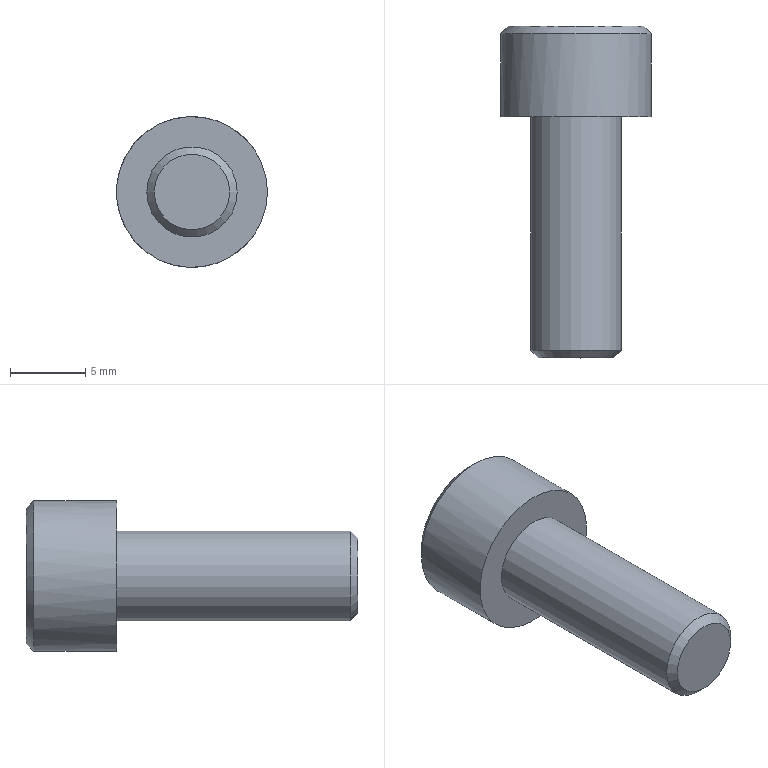Part | STEP file | gslz 2016.10.28-6_id710_x_t | 1 solid | 14 faces | box 10 x 22 x 10 mm | volume 831.004 mm3 | plane 10 | cylinder 2 | cone 2 | commonest cylinder face diameters 6 x1 10 x1
STEP:
#1=CARTESIAN_POINT('',(102.7,216.01,67.));
#2=VERTEX_POINT('',#1);
#3=CARTESIAN_POINT('',(107.2,216.01,67.));
#4=DIRECTION('',(0.000000365,1.,0.));
#5=DIRECTION('',(-1.,0.000000365,0.));
#6=AXIS2_PLACEMENT_3D('',#3,#4,#5);
#7=CIRCLE('',#6,4.5);
#8=EDGE_CURVE('',#2,#2,#7,.T.);
#9=ORIENTED_EDGE('',*,*,#8,.T.);
#10=EDGE_LOOP('',(#9));
#11=FACE_BOUND('',#10,.T.);
#12=CARTESIAN_POINT('',(109.7,216.01,68.443));
#13=VERTEX_POINT('',#12);
#14=CARTESIAN_POINT('',(109.7,216.01,65.557));
#15=VERTEX_POINT('',#14);
#16=CARTESIAN_POINT('',(109.7,216.01,68.443));
#17=DIRECTION('',(0.,0.,-1.));
#18=VECTOR('',#17,1.);
#19=LINE('',#16,#18);
#20=EDGE_CURVE('',#13,#15,#19,.T.);
#21=ORIENTED_EDGE('',*,*,#20,.F.);
#22=CARTESIAN_POINT('',(107.2,216.01,69.887));
#23=VERTEX_POINT('',#22);
#24=CARTESIAN_POINT('',(107.2,216.01,69.887));
#25=DIRECTION('',(0.866,-0.000000316,-0.5));
#26=VECTOR('',#25,1.);
#27=LINE('',#24,#26);
#28=EDGE_CURVE('',#23,#13,#27,.T.);
#29=ORIENTED_EDGE('',*,*,#28,.F.);
#30=CARTESIAN_POINT('',(104.7,216.01,68.443));
#31=VERTEX_POINT('',#30);
#32=CARTESIAN_POINT('',(104.7,216.01,68.443));
#33=DIRECTION('',(0.866,-0.000000316,0.5));
#34=VECTOR('',#33,1.);
#35=LINE('',#32,#34);
#36=EDGE_CURVE('',#31,#23,#35,.T.);
#37=ORIENTED_EDGE('',*,*,#36,.F.);
#38=CARTESIAN_POINT('',(104.7,216.01,65.557));
#39=VERTEX_POINT('',#38);
#40=CARTESIAN_POINT('',(104.7,216.01,65.557));
#41=DIRECTION('',(0.,0.,1.));
#42=VECTOR('',#41,1.);
#43=LINE('',#40,#42);
#44=EDGE_CURVE('',#39,#31,#43,.T.);
#45=ORIENTED_EDGE('',*,*,#44,.F.);
#46=CARTESIAN_POINT('',(107.2,216.01,64.113));
#47=VERTEX_POINT('',#46);
#48=CARTESIAN_POINT('',(107.2,216.01,64.113));
#49=DIRECTION('',(-0.866,0.000000316,0.5));
#50=VECTOR('',#49,1.);
#51=LINE('',#48,#50);
#52=EDGE_CURVE('',#47,#39,#51,.T.);
#53=ORIENTED_EDGE('',*,*,#52,.F.);
#54=CARTESIAN_POINT('',(109.7,216.01,65.557));
#55=DIRECTION('',(-0.866,0.000000316,-0.5));
#56=VECTOR('',#55,1.);
#57=LINE('',#54,#56);
#58=EDGE_CURVE('',#15,#47,#57,.T.);
#59=ORIENTED_EDGE('',*,*,#58,.F.);
#60=EDGE_LOOP('',(#21,#29,#37,#45,#53,#59));
#61=FACE_BOUND('',#60,.T.);
#62=CARTESIAN_POINT('',(107.2,216.01,67.));
#63=DIRECTION('',(0.000000365,1.,0.));
#64=DIRECTION('',(1.,-0.000000365,0.));
#65=AXIS2_PLACEMENT_3D('',#62,#63,#64);
#66=PLANE('',#65);
#67=ADVANCED_FACE('',(#11,#61),#66,.T.);
#68=CARTESIAN_POINT('',(109.7,194.01,67.));
#69=VERTEX_POINT('',#68);
#70=CARTESIAN_POINT('',(107.2,194.01,67.));
#71=DIRECTION('',(-0.000000365,-1.,0.));
#72=DIRECTION('',(1.,-0.000000365,0.));
#73=AXIS2_PLACEMENT_3D('',#70,#71,#72);
#74=CIRCLE('',#73,2.5);
#75=EDGE_CURVE('',#69,#69,#74,.T.);
#76=ORIENTED_EDGE('',*,*,#75,.T.);
#77=EDGE_LOOP('',(#76));
#78=FACE_OUTER_BOUND('',#77,.T.);
#79=CARTESIAN_POINT('',(107.2,194.01,67.));
#80=DIRECTION('',(-0.000000365,-1.,0.));
#81=DIRECTION('',(-1.,0.000000365,0.));
#82=AXIS2_PLACEMENT_3D('',#79,#80,#81);
#83=PLANE('',#82);
#84=ADVANCED_FACE('',(#78),#83,.T.);
#85=CARTESIAN_POINT('',(104.2,194.51,67.));
#86=VERTEX_POINT('',#85);
#87=CARTESIAN_POINT('',(107.2,194.51,67.));
#88=DIRECTION('',(0.000000365,1.,0.));
#89=DIRECTION('',(-1.,0.000000365,0.));
#90=AXIS2_PLACEMENT_3D('',#87,#88,#89);
#91=CIRCLE('',#90,3.);
#92=EDGE_CURVE('',#86,#86,#91,.T.);
#93=ORIENTED_EDGE('',*,*,#92,.T.);
#94=EDGE_LOOP('',(#93));
#95=FACE_BOUND('',#94,.T.);
#96=CARTESIAN_POINT('',(110.2,210.01,67.));
#97=VERTEX_POINT('',#96);
#98=CARTESIAN_POINT('',(107.2,210.01,67.));
#99=DIRECTION('',(-0.000000365,-1.,0.));
#100=DIRECTION('',(1.,-0.000000365,0.));
#101=AXIS2_PLACEMENT_3D('',#98,#99,#100);
#102=CIRCLE('',#101,3.);
#103=EDGE_CURVE('',#97,#97,#102,.T.);
#104=ORIENTED_EDGE('',*,*,#103,.T.);
#105=EDGE_LOOP('',(#104));
#106=FACE_BOUND('',#105,.T.);
#107=CARTESIAN_POINT('',(107.2,204.01,67.));
#108=DIRECTION('',(-0.000000365,-1.,0.));
#109=DIRECTION('',(1.,-0.000000365,0.));
#110=AXIS2_PLACEMENT_3D('',#107,#108,#109);
#111=CYLINDRICAL_SURFACE('',#110,3.);
#112=ADVANCED_FACE('',(#95,#106),#111,.T.);
#113=ORIENTED_EDGE('',*,*,#103,.F.);
#114=EDGE_LOOP('',(#113));
#115=FACE_BOUND('',#114,.T.);
#116=CARTESIAN_POINT('',(112.2,210.01,67.));
#117=VERTEX_POINT('',#116);
#118=CARTESIAN_POINT('',(107.2,210.01,67.));
#119=DIRECTION('',(-0.000000365,-1.,0.));
#120=DIRECTION('',(1.,-0.000000365,0.));
#121=AXIS2_PLACEMENT_3D('',#118,#119,#120);
#122=CIRCLE('',#121,5.);
#123=EDGE_CURVE('',#117,#117,#122,.T.);
#124=ORIENTED_EDGE('',*,*,#123,.T.);
#125=EDGE_LOOP('',(#124));
#126=FACE_BOUND('',#125,.T.);
#127=CARTESIAN_POINT('',(107.2,210.01,67.));
#128=DIRECTION('',(-0.000000365,-1.,0.));
#129=DIRECTION('',(-1.,0.000000365,0.));
#130=AXIS2_PLACEMENT_3D('',#127,#128,#129);
#131=PLANE('',#130);
#132=ADVANCED_FACE('',(#115,#126),#131,.T.);
#133=CARTESIAN_POINT('',(102.2,215.51,67.));
#134=VERTEX_POINT('',#133);
#135=CARTESIAN_POINT('',(107.2,215.51,67.));
#136=DIRECTION('',(-0.000000365,-1.,0.));
#137=DIRECTION('',(-1.,0.000000365,0.));
#138=AXIS2_PLACEMENT_3D('',#135,#136,#137);
#139=CIRCLE('',#138,5.);
#140=EDGE_CURVE('',#134,#134,#139,.T.);
#141=ORIENTED_EDGE('',*,*,#140,.T.);
#142=EDGE_LOOP('',(#141));
#143=FACE_BOUND('',#142,.T.);
#144=ORIENTED_EDGE('',*,*,#123,.F.);
#145=EDGE_LOOP('',(#144));
#146=FACE_BOUND('',#145,.T.);
#147=CARTESIAN_POINT('',(107.2,218.01,67.));
#148=DIRECTION('',(-0.000000365,-1.,0.));
#149=DIRECTION('',(1.,-0.000000365,0.));
#150=AXIS2_PLACEMENT_3D('',#147,#148,#149);
#151=CYLINDRICAL_SURFACE('',#150,5.);
#152=ADVANCED_FACE('',(#143,#146),#151,.T.);
#153=ORIENTED_EDGE('',*,*,#92,.F.);
#154=EDGE_LOOP('',(#153));
#155=FACE_BOUND('',#154,.T.);
#156=ORIENTED_EDGE('',*,*,#75,.F.);
#157=EDGE_LOOP('',(#156));
#158=FACE_BOUND('',#157,.T.);
#159=CARTESIAN_POINT('',(107.2,194.01,67.));
#160=DIRECTION('',(0.000000365,1.,0.));
#161=DIRECTION('',(-1.,0.000000365,0.));
#162=AXIS2_PLACEMENT_3D('',#159,#160,#161);
#163=CONICAL_SURFACE('',#162,2.5,45.);
#164=ADVANCED_FACE('',(#155,#158),#163,.T.);
#165=ORIENTED_EDGE('',*,*,#20,.T.);
#166=CARTESIAN_POINT('',(109.7,212.01,65.557));
#167=VERTEX_POINT('',#166);
#168=CARTESIAN_POINT('',(109.7,212.01,65.557));
#169=DIRECTION('',(-0.000000365,-1.,0.));
#170=VECTOR('',#169,1.);
#171=LINE('',#168,#170);
#172=EDGE_CURVE('',#15,#167,#171,.T.);
#173=ORIENTED_EDGE('',*,*,#172,.T.);
#174=CARTESIAN_POINT('',(109.7,212.01,68.443));
#175=VERTEX_POINT('',#174);
#176=CARTESIAN_POINT('',(109.7,212.01,68.443));
#177=DIRECTION('',(0.,0.,1.));
#178=VECTOR('',#177,1.);
#179=LINE('',#176,#178);
#180=EDGE_CURVE('',#167,#175,#179,.T.);
#181=ORIENTED_EDGE('',*,*,#180,.T.);
#182=CARTESIAN_POINT('',(109.7,212.01,68.443));
#183=DIRECTION('',(-0.000000365,-1.,0.));
#184=VECTOR('',#183,1.);
#185=LINE('',#182,#184);
#186=EDGE_CURVE('',#13,#175,#185,.T.);
#187=ORIENTED_EDGE('',*,*,#186,.F.);
#188=EDGE_LOOP('',(#165,#173,#181,#187));
#189=FACE_OUTER_BOUND('',#188,.T.);
#190=CARTESIAN_POINT('',(109.7,212.01,68.443));
#191=DIRECTION('',(1.,-0.000000365,0.));
#192=DIRECTION('',(0.000000365,1.,0.));
#193=AXIS2_PLACEMENT_3D('',#190,#191,#192);
#194=PLANE('',#193);
#195=ADVANCED_FACE('',(#189),#194,.F.);
#196=ORIENTED_EDGE('',*,*,#58,.T.);
#197=CARTESIAN_POINT('',(107.2,212.01,64.113));
#198=VERTEX_POINT('',#197);
#199=CARTESIAN_POINT('',(107.2,212.01,64.113));
#200=DIRECTION('',(-0.000000365,-1.,0.));
#201=VECTOR('',#200,1.);
#202=LINE('',#199,#201);
#203=EDGE_CURVE('',#47,#198,#202,.T.);
#204=ORIENTED_EDGE('',*,*,#203,.T.);
#205=CARTESIAN_POINT('',(109.7,212.01,65.557));
#206=DIRECTION('',(0.866,-0.000000316,0.5));
#207=VECTOR('',#206,1.);
#208=LINE('',#205,#207);
#209=EDGE_CURVE('',#198,#167,#208,.T.);
#210=ORIENTED_EDGE('',*,*,#209,.T.);
#211=ORIENTED_EDGE('',*,*,#172,.F.);
#212=EDGE_LOOP('',(#196,#204,#210,#211));
#213=FACE_OUTER_BOUND('',#212,.T.);
#214=CARTESIAN_POINT('',(109.7,212.01,65.557));
#215=DIRECTION('',(0.5,-0.000000182,-0.866));
#216=DIRECTION('',(0.866,-0.000000316,0.5));
#217=AXIS2_PLACEMENT_3D('',#214,#215,#216);
#218=PLANE('',#217);
#219=ADVANCED_FACE('',(#213),#218,.F.);
#220=ORIENTED_EDGE('',*,*,#52,.T.);
#221=CARTESIAN_POINT('',(104.7,212.01,65.557));
#222=VERTEX_POINT('',#221);
#223=CARTESIAN_POINT('',(104.7,212.01,65.557));
#224=DIRECTION('',(-0.000000365,-1.,0.));
#225=VECTOR('',#224,1.);
#226=LINE('',#223,#225);
#227=EDGE_CURVE('',#39,#222,#226,.T.);
#228=ORIENTED_EDGE('',*,*,#227,.T.);
#229=CARTESIAN_POINT('',(107.2,212.01,64.113));
#230=DIRECTION('',(0.866,-0.000000316,-0.5));
#231=VECTOR('',#230,1.);
#232=LINE('',#229,#231);
#233=EDGE_CURVE('',#222,#198,#232,.T.);
#234=ORIENTED_EDGE('',*,*,#233,.T.);
#235=ORIENTED_EDGE('',*,*,#203,.F.);
#236=EDGE_LOOP('',(#220,#228,#234,#235));
#237=FACE_OUTER_BOUND('',#236,.T.);
#238=CARTESIAN_POINT('',(107.2,212.01,64.113));
#239=DIRECTION('',(-0.5,0.000000182,-0.866));
#240=DIRECTION('',(0.866,-0.000000316,-0.5));
#241=AXIS2_PLACEMENT_3D('',#238,#239,#240);
#242=PLANE('',#241);
#243=ADVANCED_FACE('',(#237),#242,.F.);
#244=ORIENTED_EDGE('',*,*,#44,.T.);
#245=CARTESIAN_POINT('',(104.7,212.01,68.443));
#246=VERTEX_POINT('',#245);
#247=CARTESIAN_POINT('',(104.7,212.01,68.443));
#248=DIRECTION('',(-0.000000365,-1.,0.));
#249=VECTOR('',#248,1.);
#250=LINE('',#247,#249);
#251=EDGE_CURVE('',#31,#246,#250,.T.);
#252=ORIENTED_EDGE('',*,*,#251,.T.);
#253=CARTESIAN_POINT('',(104.7,212.01,65.557));
#254=DIRECTION('',(0.,0.,-1.));
#255=VECTOR('',#254,1.);
#256=LINE('',#253,#255);
#257=EDGE_CURVE('',#246,#222,#256,.T.);
#258=ORIENTED_EDGE('',*,*,#257,.T.);
#259=ORIENTED_EDGE('',*,*,#227,.F.);
#260=EDGE_LOOP('',(#244,#252,#258,#259));
#261=FACE_OUTER_BOUND('',#260,.T.);
#262=CARTESIAN_POINT('',(104.7,212.01,65.557));
#263=DIRECTION('',(-1.,0.000000365,0.));
#264=DIRECTION('',(0.000000365,1.,0.));
#265=AXIS2_PLACEMENT_3D('',#262,#263,#264);
#266=PLANE('',#265);
#267=ADVANCED_FACE('',(#261),#266,.F.);
#268=ORIENTED_EDGE('',*,*,#36,.T.);
#269=CARTESIAN_POINT('',(107.2,212.01,69.887));
#270=VERTEX_POINT('',#269);
#271=CARTESIAN_POINT('',(107.2,212.01,69.887));
#272=DIRECTION('',(-0.000000365,-1.,0.));
#273=VECTOR('',#272,1.);
#274=LINE('',#271,#273);
#275=EDGE_CURVE('',#23,#270,#274,.T.);
#276=ORIENTED_EDGE('',*,*,#275,.T.);
#277=CARTESIAN_POINT('',(104.7,212.01,68.443));
#278=DIRECTION('',(-0.866,0.000000316,-0.5));
#279=VECTOR('',#278,1.);
#280=LINE('',#277,#279);
#281=EDGE_CURVE('',#270,#246,#280,.T.);
#282=ORIENTED_EDGE('',*,*,#281,.T.);
#283=ORIENTED_EDGE('',*,*,#251,.F.);
#284=EDGE_LOOP('',(#268,#276,#282,#283));
#285=FACE_OUTER_BOUND('',#284,.T.);
#286=CARTESIAN_POINT('',(104.7,212.01,68.443));
#287=DIRECTION('',(-0.5,0.000000182,0.866));
#288=DIRECTION('',(-0.866,0.000000316,-0.5));
#289=AXIS2_PLACEMENT_3D('',#286,#287,#288);
#290=PLANE('',#289);
#291=ADVANCED_FACE('',(#285),#290,.F.);
#292=ORIENTED_EDGE('',*,*,#28,.T.);
#293=ORIENTED_EDGE('',*,*,#186,.T.);
#294=CARTESIAN_POINT('',(107.2,212.01,69.887));
#295=DIRECTION('',(-0.866,0.000000316,0.5));
#296=VECTOR('',#295,1.);
#297=LINE('',#294,#296);
#298=EDGE_CURVE('',#175,#270,#297,.T.);
#299=ORIENTED_EDGE('',*,*,#298,.T.);
#300=ORIENTED_EDGE('',*,*,#275,.F.);
#301=EDGE_LOOP('',(#292,#293,#299,#300));
#302=FACE_OUTER_BOUND('',#301,.T.);
#303=CARTESIAN_POINT('',(107.2,212.01,69.887));
#304=DIRECTION('',(0.5,-0.000000182,0.866));
#305=DIRECTION('',(-0.866,0.000000316,0.5));
#306=AXIS2_PLACEMENT_3D('',#303,#304,#305);
#307=PLANE('',#306);
#308=ADVANCED_FACE('',(#302),#307,.F.);
#309=ORIENTED_EDGE('',*,*,#180,.F.);
#310=ORIENTED_EDGE('',*,*,#209,.F.);
#311=ORIENTED_EDGE('',*,*,#233,.F.);
#312=ORIENTED_EDGE('',*,*,#257,.F.);
#313=ORIENTED_EDGE('',*,*,#281,.F.);
#314=ORIENTED_EDGE('',*,*,#298,.F.);
#315=EDGE_LOOP('',(#309,#310,#311,#312,#313,#314));
#316=FACE_OUTER_BOUND('',#315,.T.);
#317=CARTESIAN_POINT('',(109.7,212.01,65.557));
#318=DIRECTION('',(0.000000365,1.,0.));
#319=DIRECTION('',(1.,-0.000000365,0.));
#320=AXIS2_PLACEMENT_3D('',#317,#318,#319);
#321=PLANE('',#320);
#322=ADVANCED_FACE('',(#316),#321,.T.);
#323=ORIENTED_EDGE('',*,*,#8,.F.);
#324=EDGE_LOOP('',(#323));
#325=FACE_BOUND('',#324,.T.);
#326=ORIENTED_EDGE('',*,*,#140,.F.);
#327=EDGE_LOOP('',(#326));
#328=FACE_BOUND('',#327,.T.);
#329=CARTESIAN_POINT('',(107.2,215.51,67.));
#330=DIRECTION('',(-0.000000365,-1.,0.));
#331=DIRECTION('',(1.,-0.000000365,0.));
#332=AXIS2_PLACEMENT_3D('',#329,#330,#331);
#333=CONICAL_SURFACE('',#332,5.,45.);
#334=ADVANCED_FACE('',(#325,#328),#333,.T.);
#335=CLOSED_SHELL('',(#67,#84,#112,#132,#152,#164,#195,#219,#243,#267,#291,#308,#322,#334));
#336=MANIFOLD_SOLID_BREP('',#335);
#337=(LENGTH_UNIT()NAMED_UNIT(*)SI_UNIT(.MILLI.,.METRE.));
#338=UNCERTAINTY_MEASURE_WITH_UNIT(LENGTH_MEASURE(0.00002),#337,'','');
#339=(NAMED_UNIT(*)PLANE_ANGLE_UNIT()SI_UNIT($,.RADIAN.));
#340=PLANE_ANGLE_MEASURE_WITH_UNIT(PLANE_ANGLE_MEASURE(0.01745),#339);
#341=DIMENSIONAL_EXPONENTS(0.,0.,0.,0.,0.,0.,0.);
#342=(CONVERSION_BASED_UNIT('DEGREE',#340)NAMED_UNIT(#341)PLANE_ANGLE_UNIT());
#343=(NAMED_UNIT(*)SI_UNIT($,.STERADIAN.)SOLID_ANGLE_UNIT());
#344=(GEOMETRIC_REPRESENTATION_CONTEXT(3)GLOBAL_UNCERTAINTY_ASSIGNED_CONTEXT((#338))GLOBAL_UNIT_ASSIGNED_CONTEXT((#337,#342,#343))REPRESENTATION_CONTEXT('',''));
#345=ADVANCED_BREP_SHAPE_REPRESENTATION('',(#336),#344);